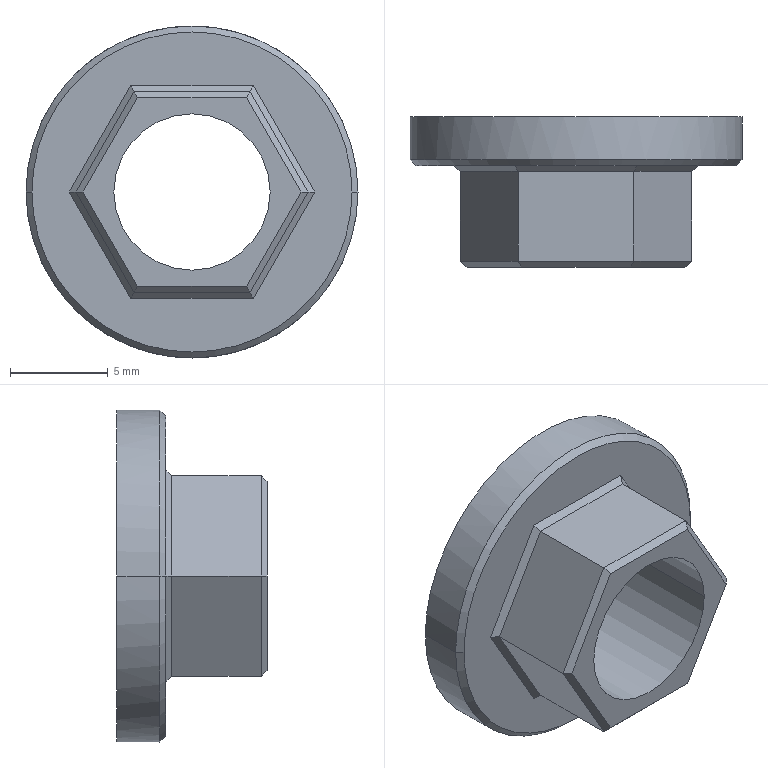Part | NX | features solid 2 | 1 solid | 27 faces | box 17 x 7.7 x 17 mm | volume 653.095 mm3 | plane 21 | cylinder 4 | cone 2 | commonest cylinder face diameters 8 x2 17 x2
STEP:
#1=CARTESIAN_POINT('',(211.5,-9.,-970.669));
#2=VERTEX_POINT('',#1);
#3=CARTESIAN_POINT('',(228.5,-9.,-970.669));
#4=VERTEX_POINT('',#3);
#5=CARTESIAN_POINT('',(220.,-9.,-970.669));
#6=DIRECTION('',(0.,-1.,0.));
#7=DIRECTION('',(-1.,0.,0.));
#8=AXIS2_PLACEMENT_3D('',#5,#6,#7);
#9=CIRCLE('',#8,8.5);
#10=EDGE_CURVE('',#2,#4,#9,.T.);
#11=ORIENTED_EDGE('',*,*,#10,.F.);
#12=CARTESIAN_POINT('',(220.,-9.,-970.669));
#13=DIRECTION('',(0.,-1.,0.));
#14=DIRECTION('',(1.,0.,0.));
#15=AXIS2_PLACEMENT_3D('',#12,#13,#14);
#16=CIRCLE('',#15,8.5);
#17=EDGE_CURVE('',#4,#2,#16,.T.);
#18=ORIENTED_EDGE('',*,*,#17,.F.);
#19=EDGE_LOOP('',(#11,#18));
#20=FACE_BOUND('',#19,.T.);
#21=CARTESIAN_POINT('',(224.,-9.,-970.669));
#22=VERTEX_POINT('',#21);
#23=CARTESIAN_POINT('',(216.,-9.,-970.669));
#24=VERTEX_POINT('',#23);
#25=CARTESIAN_POINT('',(220.,-9.,-970.669));
#26=DIRECTION('',(0.,1.,0.));
#27=DIRECTION('',(1.,0.,0.));
#28=AXIS2_PLACEMENT_3D('',#25,#26,#27);
#29=CIRCLE('',#28,4.);
#30=EDGE_CURVE('',#22,#24,#29,.T.);
#31=ORIENTED_EDGE('',*,*,#30,.F.);
#32=CARTESIAN_POINT('',(220.,-9.,-970.669));
#33=DIRECTION('',(0.,1.,0.));
#34=DIRECTION('',(-1.,0.,0.));
#35=AXIS2_PLACEMENT_3D('',#32,#33,#34);
#36=CIRCLE('',#35,4.);
#37=EDGE_CURVE('',#24,#22,#36,.T.);
#38=ORIENTED_EDGE('',*,*,#37,.F.);
#39=EDGE_LOOP('',(#31,#38));
#40=FACE_BOUND('',#39,.T.);
#41=CARTESIAN_POINT('',(220.,-9.,-970.669));
#42=DIRECTION('',(0.,-1.,0.));
#43=DIRECTION('',(-1.,0.,0.));
#44=AXIS2_PLACEMENT_3D('',#41,#42,#43);
#45=PLANE('',#44);
#46=ADVANCED_FACE('',(#20,#40),#45,.F.);
#47=CARTESIAN_POINT('',(228.5,-11.195,-970.669));
#48=VERTEX_POINT('',#47);
#49=CARTESIAN_POINT('',(228.5,-9.,-970.669));
#50=DIRECTION('',(0.,-1.,0.));
#51=VECTOR('',#50,1000.);
#52=LINE('',#49,#51);
#53=EDGE_CURVE('',#4,#48,#52,.T.);
#54=ORIENTED_EDGE('',*,*,#53,.F.);
#55=ORIENTED_EDGE('',*,*,#17,.T.);
#56=CARTESIAN_POINT('',(211.5,-11.195,-970.669));
#57=VERTEX_POINT('',#56);
#58=CARTESIAN_POINT('',(211.5,-9.,-970.669));
#59=DIRECTION('',(0.,-1.,0.));
#60=VECTOR('',#59,1000.);
#61=LINE('',#58,#60);
#62=EDGE_CURVE('',#57,#2,#61,.F.);
#63=ORIENTED_EDGE('',*,*,#62,.F.);
#64=CARTESIAN_POINT('',(220.,-11.195,-962.169));
#65=VERTEX_POINT('',#64);
#66=CARTESIAN_POINT('',(220.,-11.195,-970.669));
#67=DIRECTION('',(0.,1.,0.));
#68=DIRECTION('',(-1.,0.,0.));
#69=AXIS2_PLACEMENT_3D('',#66,#67,#68);
#70=CIRCLE('',#69,8.5);
#71=EDGE_CURVE('',#57,#65,#70,.T.);
#72=ORIENTED_EDGE('',*,*,#71,.T.);
#73=CARTESIAN_POINT('',(220.,-11.195,-970.669));
#74=DIRECTION('',(0.,1.,0.));
#75=DIRECTION('',(0.,0.,1.));
#76=AXIS2_PLACEMENT_3D('',#73,#74,#75);
#77=CIRCLE('',#76,8.5);
#78=EDGE_CURVE('',#65,#48,#77,.T.);
#79=ORIENTED_EDGE('',*,*,#78,.T.);
#80=EDGE_LOOP('',(#54,#55,#63,#72,#79));
#81=FACE_BOUND('',#80,.T.);
#82=CARTESIAN_POINT('',(220.,-9.,-970.669));
#83=DIRECTION('',(0.,-1.,0.));
#84=DIRECTION('',(-1.,0.,0.));
#85=AXIS2_PLACEMENT_3D('',#82,#83,#84);
#86=CYLINDRICAL_SURFACE('',#85,8.5);
#87=ADVANCED_FACE('',(#81),#86,.T.);
#88=CARTESIAN_POINT('',(228.195,-11.5,-970.669));
#89=VERTEX_POINT('',#88);
#90=CARTESIAN_POINT('',(228.195,-11.5,-970.669));
#91=DIRECTION('',(0.7071,0.7071,0.));
#92=VECTOR('',#91,1000.);
#93=LINE('',#90,#92);
#94=EDGE_CURVE('',#89,#48,#93,.T.);
#95=ORIENTED_EDGE('',*,*,#94,.T.);
#96=ORIENTED_EDGE('',*,*,#78,.F.);
#97=ORIENTED_EDGE('',*,*,#71,.F.);
#98=CARTESIAN_POINT('',(211.805,-11.5,-970.669));
#99=VERTEX_POINT('',#98);
#100=CARTESIAN_POINT('',(211.805,-11.5,-970.669));
#101=DIRECTION('',(-0.7071,0.7071,0.));
#102=VECTOR('',#101,1000.);
#103=LINE('',#100,#102);
#104=EDGE_CURVE('',#57,#99,#103,.F.);
#105=ORIENTED_EDGE('',*,*,#104,.T.);
#106=CARTESIAN_POINT('',(220.,-11.5,-962.474));
#107=VERTEX_POINT('',#106);
#108=CARTESIAN_POINT('',(220.,-11.5,-970.669));
#109=DIRECTION('',(0.,1.,0.));
#110=DIRECTION('',(-1.,0.,0.));
#111=AXIS2_PLACEMENT_3D('',#108,#109,#110);
#112=CIRCLE('',#111,8.195);
#113=EDGE_CURVE('',#99,#107,#112,.T.);
#114=ORIENTED_EDGE('',*,*,#113,.T.);
#115=CARTESIAN_POINT('',(220.,-11.5,-970.669));
#116=DIRECTION('',(0.,1.,0.));
#117=DIRECTION('',(0.,0.,1.));
#118=AXIS2_PLACEMENT_3D('',#115,#116,#117);
#119=CIRCLE('',#118,8.195);
#120=EDGE_CURVE('',#107,#89,#119,.T.);
#121=ORIENTED_EDGE('',*,*,#120,.T.);
#122=EDGE_LOOP('',(#95,#96,#97,#105,#114,#121));
#123=FACE_BOUND('',#122,.T.);
#124=CARTESIAN_POINT('',(220.,-11.348,-970.669));
#125=DIRECTION('',(0.,1.,0.));
#126=DIRECTION('',(0.,0.,1.));
#127=AXIS2_PLACEMENT_3D('',#124,#125,#126);
#128=CONICAL_SURFACE('',#127,8.348,0.7854);
#129=ADVANCED_FACE('',(#123),#128,.T.);
#130=CARTESIAN_POINT('',(220.,-11.5,-978.864));
#131=VERTEX_POINT('',#130);
#132=CARTESIAN_POINT('',(220.,-11.5,-970.669));
#133=DIRECTION('',(0.,1.,0.));
#134=DIRECTION('',(0.,0.,-1.));
#135=AXIS2_PLACEMENT_3D('',#132,#133,#134);
#136=CIRCLE('',#135,8.195);
#137=EDGE_CURVE('',#131,#99,#136,.T.);
#138=ORIENTED_EDGE('',*,*,#137,.F.);
#139=CARTESIAN_POINT('',(220.,-11.5,-970.669));
#140=DIRECTION('',(0.,1.,0.));
#141=DIRECTION('',(1.,0.,0.));
#142=AXIS2_PLACEMENT_3D('',#139,#140,#141);
#143=CIRCLE('',#142,8.195);
#144=EDGE_CURVE('',#89,#131,#143,.T.);
#145=ORIENTED_EDGE('',*,*,#144,.F.);
#146=ORIENTED_EDGE('',*,*,#120,.F.);
#147=ORIENTED_EDGE('',*,*,#113,.F.);
#148=EDGE_LOOP('',(#138,#145,#146,#147));
#149=FACE_BOUND('',#148,.T.);
#150=CARTESIAN_POINT('',(223.141,-11.5,-965.229));
#151=VERTEX_POINT('',#150);
#152=CARTESIAN_POINT('',(216.859,-11.5,-965.229));
#153=VERTEX_POINT('',#152);
#154=CARTESIAN_POINT('',(223.141,-11.5,-965.229));
#155=DIRECTION('',(-1.,0.,0.));
#156=VECTOR('',#155,1000.);
#157=LINE('',#154,#156);
#158=EDGE_CURVE('',#151,#153,#157,.T.);
#159=ORIENTED_EDGE('',*,*,#158,.F.);
#160=CARTESIAN_POINT('',(226.282,-11.5,-970.669));
#161=VERTEX_POINT('',#160);
#162=CARTESIAN_POINT('',(226.282,-11.5,-970.669));
#163=DIRECTION('',(-0.5,0.,0.866));
#164=VECTOR('',#163,1000.);
#165=LINE('',#162,#164);
#166=EDGE_CURVE('',#161,#151,#165,.T.);
#167=ORIENTED_EDGE('',*,*,#166,.F.);
#168=CARTESIAN_POINT('',(223.141,-11.5,-976.11));
#169=VERTEX_POINT('',#168);
#170=CARTESIAN_POINT('',(223.141,-11.5,-976.11));
#171=DIRECTION('',(0.5,0.,0.866));
#172=VECTOR('',#171,1000.);
#173=LINE('',#170,#172);
#174=EDGE_CURVE('',#169,#161,#173,.T.);
#175=ORIENTED_EDGE('',*,*,#174,.F.);
#176=CARTESIAN_POINT('',(216.859,-11.5,-976.11));
#177=VERTEX_POINT('',#176);
#178=CARTESIAN_POINT('',(216.859,-11.5,-976.11));
#179=DIRECTION('',(1.,0.,0.));
#180=VECTOR('',#179,1000.);
#181=LINE('',#178,#180);
#182=EDGE_CURVE('',#177,#169,#181,.T.);
#183=ORIENTED_EDGE('',*,*,#182,.F.);
#184=CARTESIAN_POINT('',(213.718,-11.5,-970.669));
#185=VERTEX_POINT('',#184);
#186=CARTESIAN_POINT('',(213.718,-11.5,-970.669));
#187=DIRECTION('',(0.5,0.,-0.866));
#188=VECTOR('',#187,1000.);
#189=LINE('',#186,#188);
#190=EDGE_CURVE('',#185,#177,#189,.T.);
#191=ORIENTED_EDGE('',*,*,#190,.F.);
#192=CARTESIAN_POINT('',(216.859,-11.5,-965.229));
#193=DIRECTION('',(-0.5,0.,-0.866));
#194=VECTOR('',#193,1000.);
#195=LINE('',#192,#194);
#196=EDGE_CURVE('',#153,#185,#195,.T.);
#197=ORIENTED_EDGE('',*,*,#196,.F.);
#198=EDGE_LOOP('',(#159,#167,#175,#183,#191,#197));
#199=FACE_BOUND('',#198,.T.);
#200=CARTESIAN_POINT('',(220.,-11.5,-970.669));
#201=DIRECTION('',(0.,-1.,0.));
#202=DIRECTION('',(-1.,0.,0.));
#203=AXIS2_PLACEMENT_3D('',#200,#201,#202);
#204=PLANE('',#203);
#205=ADVANCED_FACE('',(#149,#199),#204,.T.);
#206=ORIENTED_EDGE('',*,*,#104,.F.);
#207=CARTESIAN_POINT('',(220.,-11.195,-979.169));
#208=VERTEX_POINT('',#207);
#209=CARTESIAN_POINT('',(220.,-11.195,-970.669));
#210=DIRECTION('',(0.,1.,0.));
#211=DIRECTION('',(0.,0.,-1.));
#212=AXIS2_PLACEMENT_3D('',#209,#210,#211);
#213=CIRCLE('',#212,8.5);
#214=EDGE_CURVE('',#208,#57,#213,.T.);
#215=ORIENTED_EDGE('',*,*,#214,.F.);
#216=CARTESIAN_POINT('',(220.,-11.195,-970.669));
#217=DIRECTION('',(0.,1.,0.));
#218=DIRECTION('',(1.,0.,0.));
#219=AXIS2_PLACEMENT_3D('',#216,#217,#218);
#220=CIRCLE('',#219,8.5);
#221=EDGE_CURVE('',#48,#208,#220,.T.);
#222=ORIENTED_EDGE('',*,*,#221,.F.);
#223=ORIENTED_EDGE('',*,*,#94,.F.);
#224=ORIENTED_EDGE('',*,*,#144,.T.);
#225=ORIENTED_EDGE('',*,*,#137,.T.);
#226=EDGE_LOOP('',(#206,#215,#222,#223,#224,#225));
#227=FACE_BOUND('',#226,.T.);
#228=CARTESIAN_POINT('',(220.,-11.348,-970.669));
#229=DIRECTION('',(0.,1.,0.));
#230=DIRECTION('',(0.,0.,1.));
#231=AXIS2_PLACEMENT_3D('',#228,#229,#230);
#232=CONICAL_SURFACE('',#231,8.348,0.7854);
#233=ADVANCED_FACE('',(#227),#232,.T.);
#234=ORIENTED_EDGE('',*,*,#62,.T.);
#235=ORIENTED_EDGE('',*,*,#10,.T.);
#236=ORIENTED_EDGE('',*,*,#53,.T.);
#237=ORIENTED_EDGE('',*,*,#221,.T.);
#238=ORIENTED_EDGE('',*,*,#214,.T.);
#239=EDGE_LOOP('',(#234,#235,#236,#237,#238));
#240=FACE_BOUND('',#239,.T.);
#241=CARTESIAN_POINT('',(220.,-9.,-970.669));
#242=DIRECTION('',(0.,-1.,0.));
#243=DIRECTION('',(-1.,0.,0.));
#244=AXIS2_PLACEMENT_3D('',#241,#242,#243);
#245=CYLINDRICAL_SURFACE('',#244,8.5);
#246=ADVANCED_FACE('',(#240),#245,.T.);
#247=CARTESIAN_POINT('',(214.07,-11.805,-970.669));
#248=VERTEX_POINT('',#247);
#249=CARTESIAN_POINT('',(214.07,-11.805,-970.669));
#250=DIRECTION('',(-0.7559,0.6547,0.));
#251=VECTOR('',#250,1000.);
#252=LINE('',#249,#251);
#253=EDGE_CURVE('',#248,#185,#252,.T.);
#254=ORIENTED_EDGE('',*,*,#253,.F.);
#255=CARTESIAN_POINT('',(217.035,-11.805,-965.534));
#256=VERTEX_POINT('',#255);
#257=CARTESIAN_POINT('',(217.035,-11.805,-965.534));
#258=DIRECTION('',(-0.5,0.,-0.866));
#259=VECTOR('',#258,1000.);
#260=LINE('',#257,#259);
#261=EDGE_CURVE('',#256,#248,#260,.T.);
#262=ORIENTED_EDGE('',*,*,#261,.F.);
#263=CARTESIAN_POINT('',(217.035,-11.805,-965.534));
#264=DIRECTION('',(-0.378,0.6547,0.6547));
#265=VECTOR('',#264,1000.);
#266=LINE('',#263,#265);
#267=EDGE_CURVE('',#256,#153,#266,.T.);
#268=ORIENTED_EDGE('',*,*,#267,.T.);
#269=ORIENTED_EDGE('',*,*,#196,.T.);
#270=EDGE_LOOP('',(#254,#262,#268,#269));
#271=FACE_BOUND('',#270,.T.);
#272=CARTESIAN_POINT('',(215.42,-11.652,-968.025));
#273=DIRECTION('',(-0.6124,-0.7071,0.3536));
#274=DIRECTION('',(0.6124,-0.7071,-0.3536));
#275=AXIS2_PLACEMENT_3D('',#272,#273,#274);
#276=PLANE('',#275);
#277=ADVANCED_FACE('',(#271),#276,.T.);
#278=ORIENTED_EDGE('',*,*,#267,.F.);
#279=CARTESIAN_POINT('',(222.965,-11.805,-965.534));
#280=VERTEX_POINT('',#279);
#281=CARTESIAN_POINT('',(222.965,-11.805,-965.534));
#282=DIRECTION('',(-1.,0.,0.));
#283=VECTOR('',#282,1000.);
#284=LINE('',#281,#283);
#285=EDGE_CURVE('',#280,#256,#284,.T.);
#286=ORIENTED_EDGE('',*,*,#285,.F.);
#287=CARTESIAN_POINT('',(222.965,-11.805,-965.534));
#288=DIRECTION('',(0.378,0.6547,0.6547));
#289=VECTOR('',#288,1000.);
#290=LINE('',#287,#289);
#291=EDGE_CURVE('',#280,#151,#290,.T.);
#292=ORIENTED_EDGE('',*,*,#291,.T.);
#293=ORIENTED_EDGE('',*,*,#158,.T.);
#294=EDGE_LOOP('',(#278,#286,#292,#293));
#295=FACE_BOUND('',#294,.T.);
#296=CARTESIAN_POINT('',(220.,-11.652,-965.381));
#297=DIRECTION('',(0.,-0.7071,0.7071));
#298=DIRECTION('',(0.,-0.7071,-0.7071));
#299=AXIS2_PLACEMENT_3D('',#296,#297,#298);
#300=PLANE('',#299);
#301=ADVANCED_FACE('',(#295),#300,.T.);
#302=ORIENTED_EDGE('',*,*,#291,.F.);
#303=CARTESIAN_POINT('',(225.93,-11.805,-970.669));
#304=VERTEX_POINT('',#303);
#305=CARTESIAN_POINT('',(225.93,-11.805,-970.669));
#306=DIRECTION('',(-0.5,0.,0.866));
#307=VECTOR('',#306,1000.);
#308=LINE('',#305,#307);
#309=EDGE_CURVE('',#304,#280,#308,.T.);
#310=ORIENTED_EDGE('',*,*,#309,.F.);
#311=CARTESIAN_POINT('',(225.93,-11.805,-970.669));
#312=DIRECTION('',(0.7559,0.6547,0.));
#313=VECTOR('',#312,1000.);
#314=LINE('',#311,#313);
#315=EDGE_CURVE('',#304,#161,#314,.T.);
#316=ORIENTED_EDGE('',*,*,#315,.T.);
#317=ORIENTED_EDGE('',*,*,#166,.T.);
#318=EDGE_LOOP('',(#302,#310,#316,#317));
#319=FACE_BOUND('',#318,.T.);
#320=CARTESIAN_POINT('',(224.58,-11.652,-968.025));
#321=DIRECTION('',(0.6124,-0.7071,0.3536));
#322=DIRECTION('',(-0.6124,-0.7071,-0.3536));
#323=AXIS2_PLACEMENT_3D('',#320,#321,#322);
#324=PLANE('',#323);
#325=ADVANCED_FACE('',(#319),#324,.T.);
#326=ORIENTED_EDGE('',*,*,#315,.F.);
#327=CARTESIAN_POINT('',(222.965,-11.805,-975.805));
#328=VERTEX_POINT('',#327);
#329=CARTESIAN_POINT('',(222.965,-11.805,-975.805));
#330=DIRECTION('',(0.5,0.,0.866));
#331=VECTOR('',#330,1000.);
#332=LINE('',#329,#331);
#333=EDGE_CURVE('',#328,#304,#332,.T.);
#334=ORIENTED_EDGE('',*,*,#333,.F.);
#335=CARTESIAN_POINT('',(222.965,-11.805,-975.805));
#336=DIRECTION('',(0.378,0.6547,-0.6547));
#337=VECTOR('',#336,1000.);
#338=LINE('',#335,#337);
#339=EDGE_CURVE('',#328,#169,#338,.T.);
#340=ORIENTED_EDGE('',*,*,#339,.T.);
#341=ORIENTED_EDGE('',*,*,#174,.T.);
#342=EDGE_LOOP('',(#326,#334,#340,#341));
#343=FACE_BOUND('',#342,.T.);
#344=CARTESIAN_POINT('',(224.58,-11.652,-973.313));
#345=DIRECTION('',(0.6124,-0.7071,-0.3536));
#346=DIRECTION('',(-0.6124,-0.7071,0.3536));
#347=AXIS2_PLACEMENT_3D('',#344,#345,#346);
#348=PLANE('',#347);
#349=ADVANCED_FACE('',(#343),#348,.T.);
#350=ORIENTED_EDGE('',*,*,#339,.F.);
#351=CARTESIAN_POINT('',(217.035,-11.805,-975.805));
#352=VERTEX_POINT('',#351);
#353=CARTESIAN_POINT('',(217.035,-11.805,-975.805));
#354=DIRECTION('',(1.,0.,0.));
#355=VECTOR('',#354,1000.);
#356=LINE('',#353,#355);
#357=EDGE_CURVE('',#352,#328,#356,.T.);
#358=ORIENTED_EDGE('',*,*,#357,.F.);
#359=CARTESIAN_POINT('',(217.035,-11.805,-975.805));
#360=DIRECTION('',(-0.378,0.6547,-0.6547));
#361=VECTOR('',#360,1000.);
#362=LINE('',#359,#361);
#363=EDGE_CURVE('',#352,#177,#362,.T.);
#364=ORIENTED_EDGE('',*,*,#363,.T.);
#365=ORIENTED_EDGE('',*,*,#182,.T.);
#366=EDGE_LOOP('',(#350,#358,#364,#365));
#367=FACE_BOUND('',#366,.T.);
#368=CARTESIAN_POINT('',(220.,-11.652,-975.957));
#369=DIRECTION('',(0.,-0.7071,-0.7071));
#370=DIRECTION('',(0.,-0.7071,0.7071));
#371=AXIS2_PLACEMENT_3D('',#368,#369,#370);
#372=PLANE('',#371);
#373=ADVANCED_FACE('',(#367),#372,.T.);
#374=ORIENTED_EDGE('',*,*,#253,.T.);
#375=ORIENTED_EDGE('',*,*,#190,.T.);
#376=ORIENTED_EDGE('',*,*,#363,.F.);
#377=CARTESIAN_POINT('',(214.07,-11.805,-970.669));
#378=DIRECTION('',(0.5,0.,-0.866));
#379=VECTOR('',#378,1000.);
#380=LINE('',#377,#379);
#381=EDGE_CURVE('',#248,#352,#380,.T.);
#382=ORIENTED_EDGE('',*,*,#381,.F.);
#383=EDGE_LOOP('',(#374,#375,#376,#382));
#384=FACE_BOUND('',#383,.T.);
#385=CARTESIAN_POINT('',(215.42,-11.652,-973.313));
#386=DIRECTION('',(-0.6124,-0.7071,-0.3536));
#387=DIRECTION('',(0.6124,-0.7071,0.3536));
#388=AXIS2_PLACEMENT_3D('',#385,#386,#387);
#389=PLANE('',#388);
#390=ADVANCED_FACE('',(#384),#389,.T.);
#391=CARTESIAN_POINT('',(214.07,-16.395,-970.669));
#392=VERTEX_POINT('',#391);
#393=CARTESIAN_POINT('',(214.07,-11.805,-970.669));
#394=DIRECTION('',(0.,-1.,0.));
#395=VECTOR('',#394,1000.);
#396=LINE('',#393,#395);
#397=EDGE_CURVE('',#248,#392,#396,.T.);
#398=ORIENTED_EDGE('',*,*,#397,.F.);
#399=ORIENTED_EDGE('',*,*,#381,.T.);
#400=CARTESIAN_POINT('',(217.035,-16.395,-975.805));
#401=VERTEX_POINT('',#400);
#402=CARTESIAN_POINT('',(217.035,-11.805,-975.805));
#403=DIRECTION('',(0.,-1.,0.));
#404=VECTOR('',#403,1000.);
#405=LINE('',#402,#404);
#406=EDGE_CURVE('',#352,#401,#405,.T.);
#407=ORIENTED_EDGE('',*,*,#406,.T.);
#408=CARTESIAN_POINT('',(214.07,-16.395,-970.669));
#409=DIRECTION('',(0.5,0.,-0.866));
#410=VECTOR('',#409,1000.);
#411=LINE('',#408,#410);
#412=EDGE_CURVE('',#392,#401,#411,.T.);
#413=ORIENTED_EDGE('',*,*,#412,.F.);
#414=EDGE_LOOP('',(#398,#399,#407,#413));
#415=FACE_BOUND('',#414,.T.);
#416=CARTESIAN_POINT('',(214.07,-11.5,-970.669));
#417=DIRECTION('',(-0.866,0.,-0.5));
#418=DIRECTION('',(-0.5,0.,0.866));
#419=AXIS2_PLACEMENT_3D('',#416,#417,#418);
#420=PLANE('',#419);
#421=ADVANCED_FACE('',(#415),#420,.T.);
#422=CARTESIAN_POINT('',(214.422,-16.7,-970.669));
#423=VERTEX_POINT('',#422);
#424=CARTESIAN_POINT('',(214.07,-16.395,-970.669));
#425=DIRECTION('',(0.7559,-0.6547,0.));
#426=VECTOR('',#425,1000.);
#427=LINE('',#424,#426);
#428=EDGE_CURVE('',#392,#423,#427,.T.);
#429=ORIENTED_EDGE('',*,*,#428,.F.);
#430=ORIENTED_EDGE('',*,*,#412,.T.);
#431=CARTESIAN_POINT('',(217.211,-16.7,-975.5));
#432=VERTEX_POINT('',#431);
#433=CARTESIAN_POINT('',(217.035,-16.395,-975.805));
#434=DIRECTION('',(0.378,-0.6547,0.6547));
#435=VECTOR('',#434,1000.);
#436=LINE('',#433,#435);
#437=EDGE_CURVE('',#401,#432,#436,.T.);
#438=ORIENTED_EDGE('',*,*,#437,.T.);
#439=CARTESIAN_POINT('',(217.211,-16.7,-975.5));
#440=DIRECTION('',(-0.5,0.,0.866));
#441=VECTOR('',#440,1000.);
#442=LINE('',#439,#441);
#443=EDGE_CURVE('',#432,#423,#442,.T.);
#444=ORIENTED_EDGE('',*,*,#443,.T.);
#445=EDGE_LOOP('',(#429,#430,#438,#444));
#446=FACE_BOUND('',#445,.T.);
#447=CARTESIAN_POINT('',(215.685,-16.547,-973.161));
#448=DIRECTION('',(-0.6124,-0.7071,-0.3536));
#449=DIRECTION('',(0.6124,-0.7071,0.3536));
#450=AXIS2_PLACEMENT_3D('',#447,#448,#449);
#451=PLANE('',#450);
#452=ADVANCED_FACE('',(#446),#451,.T.);
#453=ORIENTED_EDGE('',*,*,#443,.F.);
#454=CARTESIAN_POINT('',(222.789,-16.7,-975.5));
#455=VERTEX_POINT('',#454);
#456=CARTESIAN_POINT('',(217.211,-16.7,-975.5));
#457=DIRECTION('',(1.,0.,0.));
#458=VECTOR('',#457,1000.);
#459=LINE('',#456,#458);
#460=EDGE_CURVE('',#432,#455,#459,.T.);
#461=ORIENTED_EDGE('',*,*,#460,.T.);
#462=CARTESIAN_POINT('',(225.578,-16.7,-970.669));
#463=VERTEX_POINT('',#462);
#464=CARTESIAN_POINT('',(225.578,-16.7,-970.669));
#465=DIRECTION('',(-0.5,0.,-0.866));
#466=VECTOR('',#465,1000.);
#467=LINE('',#464,#466);
#468=EDGE_CURVE('',#463,#455,#467,.T.);
#469=ORIENTED_EDGE('',*,*,#468,.F.);
#470=CARTESIAN_POINT('',(222.789,-16.7,-965.839));
#471=VERTEX_POINT('',#470);
#472=CARTESIAN_POINT('',(222.789,-16.7,-965.839));
#473=DIRECTION('',(0.5,0.,-0.866));
#474=VECTOR('',#473,1000.);
#475=LINE('',#472,#474);
#476=EDGE_CURVE('',#471,#463,#475,.T.);
#477=ORIENTED_EDGE('',*,*,#476,.F.);
#478=CARTESIAN_POINT('',(217.211,-16.7,-965.839));
#479=VERTEX_POINT('',#478);
#480=CARTESIAN_POINT('',(222.789,-16.7,-965.839));
#481=DIRECTION('',(-1.,0.,0.));
#482=VECTOR('',#481,1000.);
#483=LINE('',#480,#482);
#484=EDGE_CURVE('',#471,#479,#483,.T.);
#485=ORIENTED_EDGE('',*,*,#484,.T.);
#486=CARTESIAN_POINT('',(214.422,-16.7,-970.669));
#487=DIRECTION('',(0.5,0.,0.866));
#488=VECTOR('',#487,1000.);
#489=LINE('',#486,#488);
#490=EDGE_CURVE('',#423,#479,#489,.T.);
#491=ORIENTED_EDGE('',*,*,#490,.F.);
#492=EDGE_LOOP('',(#453,#461,#469,#477,#485,#491));
#493=FACE_BOUND('',#492,.T.);
#494=CARTESIAN_POINT('',(216.,-16.7,-970.669));
#495=VERTEX_POINT('',#494);
#496=CARTESIAN_POINT('',(224.,-16.7,-970.669));
#497=VERTEX_POINT('',#496);
#498=CARTESIAN_POINT('',(220.,-16.7,-970.669));
#499=DIRECTION('',(0.,-1.,0.));
#500=DIRECTION('',(-1.,0.,0.));
#501=AXIS2_PLACEMENT_3D('',#498,#499,#500);
#502=CIRCLE('',#501,4.);
#503=EDGE_CURVE('',#495,#497,#502,.T.);
#504=ORIENTED_EDGE('',*,*,#503,.F.);
#505=CARTESIAN_POINT('',(220.,-16.7,-970.669));
#506=DIRECTION('',(0.,-1.,0.));
#507=DIRECTION('',(1.,0.,0.));
#508=AXIS2_PLACEMENT_3D('',#505,#506,#507);
#509=CIRCLE('',#508,4.);
#510=EDGE_CURVE('',#497,#495,#509,.T.);
#511=ORIENTED_EDGE('',*,*,#510,.F.);
#512=EDGE_LOOP('',(#504,#511));
#513=FACE_BOUND('',#512,.T.);
#514=CARTESIAN_POINT('',(220.,-16.7,-970.669));
#515=DIRECTION('',(0.,-1.,0.));
#516=DIRECTION('',(-1.,0.,0.));
#517=AXIS2_PLACEMENT_3D('',#514,#515,#516);
#518=PLANE('',#517);
#519=ADVANCED_FACE('',(#493,#513),#518,.T.);
#520=ORIENTED_EDGE('',*,*,#428,.T.);
#521=ORIENTED_EDGE('',*,*,#490,.T.);
#522=CARTESIAN_POINT('',(217.035,-16.395,-965.534));
#523=VERTEX_POINT('',#522);
#524=CARTESIAN_POINT('',(217.035,-16.395,-965.534));
#525=DIRECTION('',(0.378,-0.6547,-0.6547));
#526=VECTOR('',#525,1000.);
#527=LINE('',#524,#526);
#528=EDGE_CURVE('',#523,#479,#527,.T.);
#529=ORIENTED_EDGE('',*,*,#528,.F.);
#530=CARTESIAN_POINT('',(217.035,-16.395,-965.534));
#531=DIRECTION('',(-0.5,0.,-0.866));
#532=VECTOR('',#531,1000.);
#533=LINE('',#530,#532);
#534=EDGE_CURVE('',#523,#392,#533,.T.);
#535=ORIENTED_EDGE('',*,*,#534,.T.);
#536=EDGE_LOOP('',(#520,#521,#529,#535));
#537=FACE_BOUND('',#536,.T.);
#538=CARTESIAN_POINT('',(215.685,-16.547,-968.178));
#539=DIRECTION('',(-0.6124,-0.7071,0.3536));
#540=DIRECTION('',(0.6124,-0.7071,-0.3536));
#541=AXIS2_PLACEMENT_3D('',#538,#539,#540);
#542=PLANE('',#541);
#543=ADVANCED_FACE('',(#537),#542,.T.);
#544=CARTESIAN_POINT('',(217.035,-11.805,-965.534));
#545=DIRECTION('',(0.,-1.,0.));
#546=VECTOR('',#545,1000.);
#547=LINE('',#544,#546);
#548=EDGE_CURVE('',#256,#523,#547,.T.);
#549=ORIENTED_EDGE('',*,*,#548,.F.);
#550=ORIENTED_EDGE('',*,*,#261,.T.);
#551=ORIENTED_EDGE('',*,*,#397,.T.);
#552=ORIENTED_EDGE('',*,*,#534,.F.);
#553=EDGE_LOOP('',(#549,#550,#551,#552));
#554=FACE_BOUND('',#553,.T.);
#555=CARTESIAN_POINT('',(217.035,-11.5,-965.534));
#556=DIRECTION('',(-0.866,0.,0.5));
#557=DIRECTION('',(0.5,0.,0.866));
#558=AXIS2_PLACEMENT_3D('',#555,#556,#557);
#559=PLANE('',#558);
#560=ADVANCED_FACE('',(#554),#559,.T.);
#561=CARTESIAN_POINT('',(222.965,-16.395,-965.534));
#562=VERTEX_POINT('',#561);
#563=CARTESIAN_POINT('',(222.965,-11.805,-965.534));
#564=DIRECTION('',(0.,-1.,0.));
#565=VECTOR('',#564,1000.);
#566=LINE('',#563,#565);
#567=EDGE_CURVE('',#280,#562,#566,.T.);
#568=ORIENTED_EDGE('',*,*,#567,.F.);
#569=ORIENTED_EDGE('',*,*,#285,.T.);
#570=ORIENTED_EDGE('',*,*,#548,.T.);
#571=CARTESIAN_POINT('',(222.965,-16.395,-965.534));
#572=DIRECTION('',(-1.,0.,0.));
#573=VECTOR('',#572,1000.);
#574=LINE('',#571,#573);
#575=EDGE_CURVE('',#562,#523,#574,.T.);
#576=ORIENTED_EDGE('',*,*,#575,.F.);
#577=EDGE_LOOP('',(#568,#569,#570,#576));
#578=FACE_BOUND('',#577,.T.);
#579=CARTESIAN_POINT('',(222.965,-11.5,-965.534));
#580=DIRECTION('',(0.,0.,1.));
#581=DIRECTION('',(1.,0.,0.));
#582=AXIS2_PLACEMENT_3D('',#579,#580,#581);
#583=PLANE('',#582);
#584=ADVANCED_FACE('',(#578),#583,.T.);
#585=ORIENTED_EDGE('',*,*,#528,.T.);
#586=ORIENTED_EDGE('',*,*,#484,.F.);
#587=CARTESIAN_POINT('',(222.965,-16.395,-965.534));
#588=DIRECTION('',(-0.378,-0.6547,-0.6547));
#589=VECTOR('',#588,1000.);
#590=LINE('',#587,#589);
#591=EDGE_CURVE('',#562,#471,#590,.T.);
#592=ORIENTED_EDGE('',*,*,#591,.F.);
#593=ORIENTED_EDGE('',*,*,#575,.T.);
#594=EDGE_LOOP('',(#585,#586,#592,#593));
#595=FACE_BOUND('',#594,.T.);
#596=CARTESIAN_POINT('',(220.,-16.547,-965.686));
#597=DIRECTION('',(0.,-0.7071,0.7071));
#598=DIRECTION('',(0.,-0.7071,-0.7071));
#599=AXIS2_PLACEMENT_3D('',#596,#597,#598);
#600=PLANE('',#599);
#601=ADVANCED_FACE('',(#595),#600,.T.);
#602=ORIENTED_EDGE('',*,*,#591,.T.);
#603=ORIENTED_EDGE('',*,*,#476,.T.);
#604=CARTESIAN_POINT('',(225.93,-16.395,-970.669));
#605=VERTEX_POINT('',#604);
#606=CARTESIAN_POINT('',(225.93,-16.395,-970.669));
#607=DIRECTION('',(-0.7559,-0.6547,0.));
#608=VECTOR('',#607,1000.);
#609=LINE('',#606,#608);
#610=EDGE_CURVE('',#605,#463,#609,.T.);
#611=ORIENTED_EDGE('',*,*,#610,.F.);
#612=CARTESIAN_POINT('',(225.93,-16.395,-970.669));
#613=DIRECTION('',(-0.5,0.,0.866));
#614=VECTOR('',#613,1000.);
#615=LINE('',#612,#614);
#616=EDGE_CURVE('',#605,#562,#615,.T.);
#617=ORIENTED_EDGE('',*,*,#616,.T.);
#618=EDGE_LOOP('',(#602,#603,#611,#617));
#619=FACE_BOUND('',#618,.T.);
#620=CARTESIAN_POINT('',(224.315,-16.547,-968.178));
#621=DIRECTION('',(0.6124,-0.7071,0.3536));
#622=DIRECTION('',(-0.6124,-0.7071,-0.3536));
#623=AXIS2_PLACEMENT_3D('',#620,#621,#622);
#624=PLANE('',#623);
#625=ADVANCED_FACE('',(#619),#624,.T.);
#626=CARTESIAN_POINT('',(225.93,-11.805,-970.669));
#627=DIRECTION('',(0.,-1.,0.));
#628=VECTOR('',#627,1000.);
#629=LINE('',#626,#628);
#630=EDGE_CURVE('',#304,#605,#629,.T.);
#631=ORIENTED_EDGE('',*,*,#630,.F.);
#632=ORIENTED_EDGE('',*,*,#309,.T.);
#633=ORIENTED_EDGE('',*,*,#567,.T.);
#634=ORIENTED_EDGE('',*,*,#616,.F.);
#635=EDGE_LOOP('',(#631,#632,#633,#634));
#636=FACE_BOUND('',#635,.T.);
#637=CARTESIAN_POINT('',(225.93,-11.5,-970.669));
#638=DIRECTION('',(0.866,0.,0.5));
#639=DIRECTION('',(0.5,0.,-0.866));
#640=AXIS2_PLACEMENT_3D('',#637,#638,#639);
#641=PLANE('',#640);
#642=ADVANCED_FACE('',(#636),#641,.T.);
#643=CARTESIAN_POINT('',(222.965,-16.395,-975.805));
#644=VERTEX_POINT('',#643);
#645=CARTESIAN_POINT('',(222.965,-11.805,-975.805));
#646=DIRECTION('',(0.,-1.,0.));
#647=VECTOR('',#646,1000.);
#648=LINE('',#645,#647);
#649=EDGE_CURVE('',#328,#644,#648,.T.);
#650=ORIENTED_EDGE('',*,*,#649,.F.);
#651=ORIENTED_EDGE('',*,*,#333,.T.);
#652=ORIENTED_EDGE('',*,*,#630,.T.);
#653=CARTESIAN_POINT('',(222.965,-16.395,-975.805));
#654=DIRECTION('',(0.5,0.,0.866));
#655=VECTOR('',#654,1000.);
#656=LINE('',#653,#655);
#657=EDGE_CURVE('',#644,#605,#656,.T.);
#658=ORIENTED_EDGE('',*,*,#657,.F.);
#659=EDGE_LOOP('',(#650,#651,#652,#658));
#660=FACE_BOUND('',#659,.T.);
#661=CARTESIAN_POINT('',(222.965,-11.5,-975.805));
#662=DIRECTION('',(0.866,0.,-0.5));
#663=DIRECTION('',(-0.5,0.,-0.866));
#664=AXIS2_PLACEMENT_3D('',#661,#662,#663);
#665=PLANE('',#664);
#666=ADVANCED_FACE('',(#660),#665,.T.);
#667=ORIENTED_EDGE('',*,*,#610,.T.);
#668=ORIENTED_EDGE('',*,*,#468,.T.);
#669=CARTESIAN_POINT('',(222.965,-16.395,-975.805));
#670=DIRECTION('',(-0.378,-0.6547,0.6547));
#671=VECTOR('',#670,1000.);
#672=LINE('',#669,#671);
#673=EDGE_CURVE('',#644,#455,#672,.T.);
#674=ORIENTED_EDGE('',*,*,#673,.F.);
#675=ORIENTED_EDGE('',*,*,#657,.T.);
#676=EDGE_LOOP('',(#667,#668,#674,#675));
#677=FACE_BOUND('',#676,.T.);
#678=CARTESIAN_POINT('',(224.315,-16.547,-973.161));
#679=DIRECTION('',(0.6124,-0.7071,-0.3536));
#680=DIRECTION('',(-0.6124,-0.7071,0.3536));
#681=AXIS2_PLACEMENT_3D('',#678,#679,#680);
#682=PLANE('',#681);
#683=ADVANCED_FACE('',(#677),#682,.T.);
#684=ORIENTED_EDGE('',*,*,#673,.T.);
#685=ORIENTED_EDGE('',*,*,#460,.F.);
#686=ORIENTED_EDGE('',*,*,#437,.F.);
#687=CARTESIAN_POINT('',(217.035,-16.395,-975.805));
#688=DIRECTION('',(1.,0.,0.));
#689=VECTOR('',#688,1000.);
#690=LINE('',#687,#689);
#691=EDGE_CURVE('',#401,#644,#690,.T.);
#692=ORIENTED_EDGE('',*,*,#691,.T.);
#693=EDGE_LOOP('',(#684,#685,#686,#692));
#694=FACE_BOUND('',#693,.T.);
#695=CARTESIAN_POINT('',(220.,-16.547,-975.652));
#696=DIRECTION('',(0.,-0.7071,-0.7071));
#697=DIRECTION('',(0.,-0.7071,0.7071));
#698=AXIS2_PLACEMENT_3D('',#695,#696,#697);
#699=PLANE('',#698);
#700=ADVANCED_FACE('',(#694),#699,.T.);
#701=ORIENTED_EDGE('',*,*,#406,.F.);
#702=ORIENTED_EDGE('',*,*,#357,.T.);
#703=ORIENTED_EDGE('',*,*,#649,.T.);
#704=ORIENTED_EDGE('',*,*,#691,.F.);
#705=EDGE_LOOP('',(#701,#702,#703,#704));
#706=FACE_BOUND('',#705,.T.);
#707=CARTESIAN_POINT('',(217.035,-11.5,-975.805));
#708=DIRECTION('',(0.,0.,-1.));
#709=DIRECTION('',(-1.,0.,0.));
#710=AXIS2_PLACEMENT_3D('',#707,#708,#709);
#711=PLANE('',#710);
#712=ADVANCED_FACE('',(#706),#711,.T.);
#713=CARTESIAN_POINT('',(224.,-16.7,-970.669));
#714=DIRECTION('',(0.,1.,0.));
#715=VECTOR('',#714,1000.);
#716=LINE('',#713,#715);
#717=EDGE_CURVE('',#497,#22,#716,.T.);
#718=ORIENTED_EDGE('',*,*,#717,.F.);
#719=ORIENTED_EDGE('',*,*,#510,.T.);
#720=CARTESIAN_POINT('',(216.,-16.7,-970.669));
#721=DIRECTION('',(0.,1.,0.));
#722=VECTOR('',#721,1000.);
#723=LINE('',#720,#722);
#724=EDGE_CURVE('',#24,#495,#723,.F.);
#725=ORIENTED_EDGE('',*,*,#724,.F.);
#726=ORIENTED_EDGE('',*,*,#37,.T.);
#727=EDGE_LOOP('',(#718,#719,#725,#726));
#728=FACE_BOUND('',#727,.T.);
#729=CARTESIAN_POINT('',(220.,-16.7,-970.669));
#730=DIRECTION('',(0.,-1.,0.));
#731=DIRECTION('',(-1.,0.,0.));
#732=AXIS2_PLACEMENT_3D('',#729,#730,#731);
#733=CYLINDRICAL_SURFACE('',#732,4.);
#734=ADVANCED_FACE('',(#728),#733,.F.);
#735=ORIENTED_EDGE('',*,*,#724,.T.);
#736=ORIENTED_EDGE('',*,*,#503,.T.);
#737=ORIENTED_EDGE('',*,*,#717,.T.);
#738=ORIENTED_EDGE('',*,*,#30,.T.);
#739=EDGE_LOOP('',(#735,#736,#737,#738));
#740=FACE_BOUND('',#739,.T.);
#741=CARTESIAN_POINT('',(220.,-16.7,-970.669));
#742=DIRECTION('',(0.,-1.,0.));
#743=DIRECTION('',(-1.,0.,0.));
#744=AXIS2_PLACEMENT_3D('',#741,#742,#743);
#745=CYLINDRICAL_SURFACE('',#744,4.);
#746=ADVANCED_FACE('',(#740),#745,.F.);
#747=CLOSED_SHELL('',(#46,#87,#129,#205,#233,#246,#277,#301,#325,#349,#373,#390,#421,#452,#519,#543,#560,#584,#601,#625,#642,#666,#683,#700,#712,#734,#746));
#748=MANIFOLD_SOLID_BREP('',#747);
#749=(LENGTH_UNIT()NAMED_UNIT(*)SI_UNIT(.MILLI.,.METRE.));
#750=UNCERTAINTY_MEASURE_WITH_UNIT(LENGTH_MEASURE(0.00001),#749,'','');
#751=(NAMED_UNIT(*)PLANE_ANGLE_UNIT()SI_UNIT($,.RADIAN.));
#752=(NAMED_UNIT(*)SI_UNIT($,.STERADIAN.)SOLID_ANGLE_UNIT());
#753=(GEOMETRIC_REPRESENTATION_CONTEXT(3)GLOBAL_UNCERTAINTY_ASSIGNED_CONTEXT((#750))GLOBAL_UNIT_ASSIGNED_CONTEXT((#749,#751,#752))REPRESENTATION_CONTEXT('',''));
#754=ADVANCED_BREP_SHAPE_REPRESENTATION('',(#748),#753);